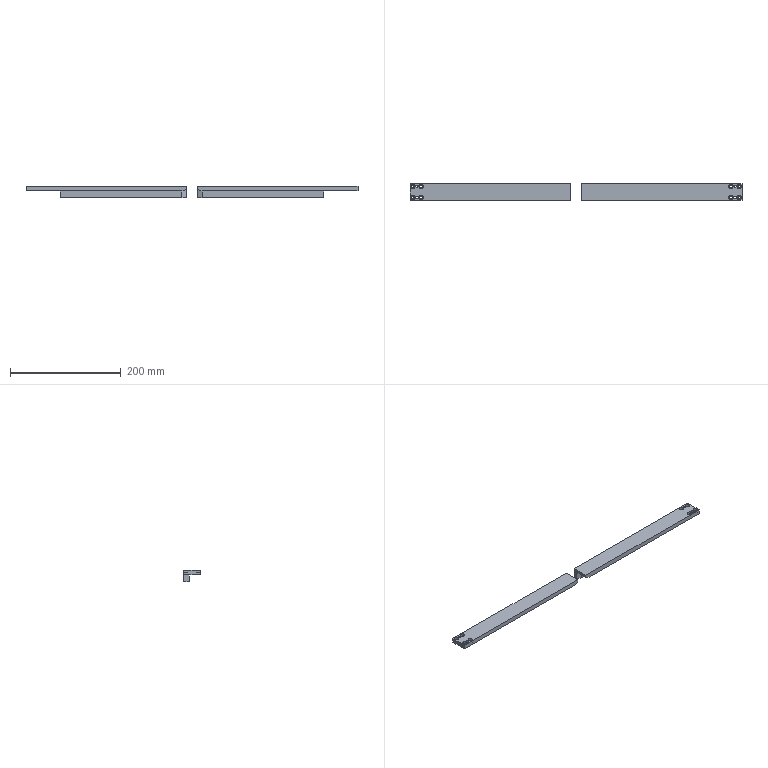NC program | NX | posted with a generic post | part box 600 x 30 x 20 mm
Whole program:
N10 G17 G21 G94 G90
(FLOOR_WALL_COPY , TOOL : D50)
N12 T01 M6
N14 G54
N16 G17 G0 G90 X-173. Y0. S6500 M3
N18 G43 Z30. H1
N20 Z7.
N22 G94 G1 Z4. F1250.
N24 X-170.
N26 X170.
N28 X173.
N30 Z7.
N32 G0 Z30.
N34 X-173.
N36 Z6.
N38 G1 Z3.
N40 X-170.
N42 X170.
N44 X173.
N46 Z6.
N48 G0 Z30.
N50 X-173.
N52 Z5.
N54 G1 Z2.
N56 X-170.
N58 X170.
N60 X173.
N62 Z5.
N64 G0 Z30.
N66 X-173.
N68 Z4.
N70 G1 Z1.
N72 X-170.
N74 X170.
N76 X173.
N78 Z4.
N80 G0 Z30.
N82 X-173.
N84 Z3.
N86 G1 Z0.
N88 X-170.
N90 X170.
N92 X173.
N94 Z3.
N96 G0 Z30.
N98 M5
(FLOOR_WALL_1 , TOOL : D10)
N100 T03 M6
N102 G54
N104 G17 G0 G90 X153.147 Y-14.991 S7000 M3
N106 G43 Z30. H3
N108 Z-8.85
N110 G94 G1 Z-11.85 F1000.
N112 X150.978
N114 X150.147 Y-17.873
N116 G2 X149.446 Y-20.147 R64. F3000.
N118 G1 X148.392
N120 G3 X150.147 Y-13.829 R63.
N122 G1 Y-8.032
N124 G2 X147.337 Y-20.147 R62.
N126 G1 X146.279
N128 G3 X149.65 Y-0.15 R61.
N130 G1 Y20.147
N132 X148.65
N134 Y-0.15
N136 G2 X145.22 Y-20.147 R60.
N138 G1 X144.158
N140 G3 X147.65 Y-0.15 R59.
N142 G1 Y20.147
N144 X146.65
N146 Y-0.15
N148 G2 X143.094 Y-20.147 R58.
N150 G1 X142.027
N152 G3 X145.65 Y-0.15 R57.
N154 G1 Y20.147
N156 X144.65
N158 Y-0.15
N160 G2 X140.958 Y-20.147 R56.
N162 G1 X139.886
N164 G3 X143.65 Y-0.15 R55.
N166 G1 Y20.147
N168 X142.65
N170 Y-0.15
N172 G2 X138.811 Y-20.147 R54.
N174 G1 X137.733
N176 G3 X141.65 Y-0.15 R53.
N178 G1 Y20.147
N180 X140.65
N182 Y-0.15
N184 G2 X136.651 Y-20.147 R52.
N186 G1 X135.566
N188 G3 X139.65 Y-0.15 R51.
N190 G1 Y20.147
N192 X138.65
N194 Y-0.15
N196 G2 X134.477 Y-20.147 R50.
N198 G1 X133.384
N200 G3 X137.65 Y-0.15 R49.
N202 G1 Y20.147
N204 X136.65
N206 Y-0.15
N208 G2 X132.286 Y-20.147 R48.
N210 G1 X131.184
N212 G3 X135.65 Y-0.15 R47.
N214 G1 Y20.147
N216 X134.65
N218 Y-0.15
N220 G2 X130.076 Y-20.147 R46.
N222 G1 X128.963
N224 G3 X133.65 Y-0.15 R45.
N226 G1 Y20.147
N228 X132.65
N230 Y-0.15
N232 G2 X127.843 Y-20.147 R44.
N234 G1 X126.717
N236 G3 X131.65 Y-0.15 R43.
N238 G1 Y20.147
N240 X130.65
N242 Y-0.15
N244 G2 X125.584 Y-20.147 R42.
N246 G1 X124.443
N248 G3 X129.65 Y-0.15 R41.
N250 G1 Y20.147
N252 X128.65
N254 Y-0.15
N256 G2 X123.293 Y-20.147 R40.
N258 G1 X122.133
N260 G3 X127.65 Y-0.15 R39.
N262 G1 Y20.147
N264 X126.65
N266 Y-0.15
N268 G2 X120.963 Y-20.147 R38.
N270 G1 X119.781
N272 G3 X125.65 Y-0.15 R37.
N274 G1 Y20.147
N276 X124.65
N278 Y-0.15
N280 G2 X118.585 Y-20.147 R36.
N282 G1 X117.375
N284 G3 X123.65 Y-0.15 R35.
N286 G1 Y20.147
N288 X122.65
N290 Y-0.15
N292 G2 X116.148 Y-20.147 R34.
N294 G1 X114.901
N296 G3 X121.65 Y-0.15 R33.
N298 G1 Y20.147
N300 X120.65
N302 Y-0.15
N304 G2 X113.632 Y-20.147 R32.
N306 G1 X112.338
N308 G3 X119.65 Y-0.15 R31.
N310 G1 Y20.147
N312 X118.65
N314 Y-0.15
N316 G2 X111.013 Y-20.147 R30.
N318 G1 X109.653
N320 G3 X117.65 Y-0.15 R29.
N322 G1 Y20.147
N324 X116.65
N326 Y-0.15
N328 G2 X108.249 Y-20.147 R28.
N330 G1 X106.792
N332 G3 X115.65 Y-0.15 R27.
N334 G1 Y20.147
N336 X114.65
N338 Y-0.15
N340 G2 X105.267 Y-20.147 R26.
N342 G1 X103.654
N344 G3 X113.65 Y-0.15 R25.
N346 G1 Y20.147
N348 X112.65
N350 Y-0.15
N352 G2 X101.921 Y-20.147 R24.
N354 G1 X100.013
N356 G3 X111.65 Y-0.15 R23.
N358 G1 Y20.147
N360 X110.65
N362 Y-0.15
N364 G2 X97.822 Y-20.147 R22.
N366 G1 X95.062
N368 G3 X109.65 Y-0.15 R21.
N370 G1 Y20.147
N372 X108.65
N374 Y-0.15
N376 G2 X88.996 Y-20.147 R20.
N378 G1 X85.997 Y-20.199
N380 Y-23.147
N382 Z-8.85
N384 G0 Z30.
N386 X-153.147 Y-18.991
N388 Z-8.85
N390 G1 Z-11.85 F1000.
N392 X-150.147 Y-20.083
N394 X-149.972 Y-20.147 F3000.
N396 X-147.048
N398 X-150.147 Y-19.019
N400 Y-17.955
N402 X-144.848 Y-19.884
N404 G3 X-144.078 Y-20.147 R21.
N406 G1 X-138.012
N408 G2 X-144.506 Y-18.944 R20.
N410 G1 X-150.147 Y-16.891
N412 Y-15.827
N414 X-144.164 Y-18.004
N416 G3 X-137.666 Y-19.15 R19.
N418 G1 X88.65
N420 G3 X107.65 Y-0.15 R19.
N422 G1 Y20.147
N424 X106.65
N426 Y-0.15
N428 G2 X88.65 Y-18.15 R18.
N430 G1 X-137.666
N432 G2 X-143.822 Y-17.064 R18.
N434 G1 X-150.147 Y-14.762
N436 Y-13.698
N438 X-143.48 Y-16.125
N440 G3 X-137.666 Y-17.15 R17.
N442 G1 X88.65
N444 G3 X105.65 Y-0.15 R17.
N446 G1 Y20.147
N448 X104.65
N450 Y-0.15
N452 G2 X88.65 Y-16.15 R16.
N454 G1 X-137.666
N456 G2 X-143.138 Y-15.185 R16.
N458 G1 X-150.147 Y-12.634
N460 Y-11.57
N462 X-142.796 Y-14.245
N464 G3 X-137.666 Y-15.15 R15.
N466 G1 X88.65
N468 G3 X103.65 Y-0.15 R15.
N470 G1 Y20.147
N472 X102.65
N474 Y-0.15
N476 G2 X88.65 Y-14.15 R14.
N478 G1 X-137.666
N480 G2 X-142.454 Y-13.306 R14.
N482 G1 X-150.147 Y-10.506
N484 Y-9.441
N486 X-142.112 Y-12.366
N488 G3 X-137.666 Y-13.15 R13.
N490 G1 X88.65
N492 G3 X101.65 Y-0.15 R13.
N494 G1 Y20.147
N496 X100.65
N498 Y-0.15
N500 G2 X88.65 Y-12.15 R12.
N502 G1 X-137.666
N504 G2 X-141.77 Y-11.426 R12.
N506 G1 X-150.147 Y-8.377
N508 Y-7.313
N510 X-141.428 Y-10.487
N512 G3 X-137.666 Y-11.15 R11.
N514 G1 X88.65
N516 G3 X99.65 Y-0.15 R11.
N518 G1 Y20.147
N520 X98.65
N522 Y-0.15
N524 G2 X88.65 Y-10.15 R10.
N526 G1 X-137.666
N528 G2 X-141.086 Y-9.547 R10.
N530 G1 X-150.147 Y-6.249
N532 Y-5.185
N534 X-140.744 Y-8.607
N536 G3 X-137.666 Y-9.15 R9.
N538 G1 X88.65
N540 G3 X97.65 Y-0.15 R9.
N542 G1 Y20.147
N544 X96.65
N546 Y-0.15
N548 G2 X88.65 Y-8.15 R8.
N550 G1 X-137.666
N552 G2 X-140.402 Y-7.668 R8.
N554 G1 X-150.147 Y-4.121
N556 Y-3.056
N558 X-140.06 Y-6.728
N560 G3 X-137.666 Y-7.15 R7.
N562 G1 X88.65
N564 G3 X95.65 Y-0.15 R7.
N566 G1 Y20.147
N568 X94.65
N570 Y-0.15
N572 G2 X88.65 Y-6.15 R6.
N574 G1 X-137.666
N576 G2 X-139.718 Y-5.788 R6.
N578 G1 X-150.147 Y-1.992
N580 Y-0.928
N582 X-139.376 Y-4.848
N584 G3 X-137.666 Y-5.15 R5.
N586 G1 X88.65
N588 G3 X93.65 Y-0.15 R5.
N590 G1 Y20.147
N592 X92.65
N594 Y-0.15
N596 G2 X88.65 Y-4.15 R4.
N598 G1 X-137.666
N600 G2 X-139.034 Y-3.909 R4.
N602 G1 X-150.147 Y0.136
N604 Y1.2
N606 X-138.692 Y-2.969
N608 G3 X-137.666 Y-3.15 R3.
N610 G1 X88.65
N612 G3 X91.65 Y-0.15 R3.
N614 G1 Y20.147
N616 X90.65
N618 Y-0.15
N620 G2 X88.65 Y-2.15 R2.
N622 G1 X-137.666
N624 G2 X-138.35 Y-2.029 R2.
N626 G1 X-150.147 Y2.264
N628 Y3.329
N630 X-138.008 Y-1.09
N632 G3 X-137.666 Y-1.15 R1.
N634 G1 X88.65
N636 G3 X89.65 Y-0.15 R1.
N638 G1 Y20.147
N640 X88.65
N642 Y-0.15
N644 X-137.666
N646 X-150.147 Y4.393
N648 X-153.15 Y5.486
N650 Z-8.85
N652 G0 Z30.
N654 M5
(FLOOR_WALL_1_COPY_1 , TOOL : D10JING)
N656 T04 M6
N658 G54
N660 G17 G0 G90 X151.139 Y-20.974 S7000 M3
N662 G43 Z30. H4
N664 Z-10.5
N666 G94 G1 Z-12. F1000.
N668 X150.865 Y-20.499
N670 G3 X149.999 Y-19.999 R1.
N672 G1 X-149.999
N674 Y-15.571
N676 X149.999
N678 Y-11.142
N680 X-149.999
N682 Y-6.714
N684 X149.999
N686 Y-2.286
N688 X-149.999
N690 Y2.142
N692 X-144.987
N694 Z-10.5
N696 G0 Z30.
N698 X94.971 Y19.999
N700 Z-10.4
N702 G1 X89. Z-12.
N704 Y2.142
N706 X149.999
N708 Y6.571
N710 X89.
N712 Y10.999
N714 X149.999
N716 Y15.427
N718 X89.
N720 G3 X89.5 Y14.561 R1.
N722 G1 Z-10.5
N724 G0 Z-8.9
N726 G1 X90.098 Y21.499 F6000.
N728 G0 Z-10.5
N730 G1 Z-12. F1000.
N732 X89. Y20.865
N734 G3 X88.5 Y19.999 R1.
N736 G1 Y0.
N738 X-137.639
N740 X-149.999 Y4.499
N742 G3 X-150.984 Y4.325 R1.
N744 G1 X-151.5 Y3.892
N746 Z-10.5
N748 G0 Z30.
N750 M5
(ZLEVEL_PROFILE_COPY_COPY_1_COPY_COPY_COPY_1_COPY_COPY , TOOL : D6R0.5)
N752 T20 M6
N754 G54
N756 G17 G0 G90 X-139.958 Y-16.121 S7000 M3
N758 G43 Z30. H20
N760 Z-12.034
N762 G94 G1 X-139.738 Y-15.994 F1000.
N764 G3 X-139.439 Y-15.474 R0.6
N766 G1 X-139.44 Y-15. F3000.
N768 Y2.784
N770 X-139.534 Y2.818 Z-12.068
N772 Y-15.
N774 X-139.533 Y-15.474
N776 X-139.581 Y-15.475 Z-12.086
N778 X-139.627 Z-12.103
N780 X-139.628 Y-15.
N782 Y2.852
N784 X-139.722 Y2.886 Z-12.137
N786 Y-15.
N788 X-139.721 Y-15.476
N790 X-139.769 Z-12.154
N792 X-139.815 Z-12.171
N794 X-139.816 Y-15.
N796 Y2.92
N798 X-139.91 Y2.955 Z-12.205
N800 Y-15.
N802 X-139.909 Y-15.477
N804 X-139.957 Z-12.222
N806 X-140.003 Z-12.239
N808 X-140.004 Y-15.
N810 Y2.989
N812 X-140.097 Y3.023 Z-12.274
N814 Y-15.
N816 Y-15.478
N818 X-140.144 Z-12.291
N820 X-140.191 Y-15.479 Z-12.308
N822 Y-15.
N824 Y3.057
N826 X-140.285 Y3.092 Z-12.342
N828 Y-15.
N830 Y-15.479
N832 X-140.332 Y-15.48 Z-12.359
N834 X-140.379 Z-12.376
N836 Y-15.
N838 Y3.126
N840 X-140.473 Y3.16 Z-12.41
N842 Y-15.
N844 Y-15.48
N846 X-140.52 Y-15.481 Z-12.428
N848 X-140.567 Z-12.445
N850 Y-15.
N852 Y3.194
N854 X-140.661 Y3.228 Z-12.479
N856 Y-15.
N858 Y-15.482
N860 X-140.708 Z-12.496
N862 X-140.755 Z-12.513
N864 Y-15.
N866 Y3.263
N868 X-140.849 Y3.297 Z-12.547
N870 Y-15.
N872 Y-15.483
N874 X-140.896 Z-12.564
N876 X-140.943 Y-15.484 Z-12.581
N878 Y-15.
N880 Y3.331
N882 X-141.037 Y3.365 Z-12.616
N884 Y-15.
N886 Y-15.484
N888 X-141.084 Z-12.633
N890 X-141.131 Y-15.485 Z-12.65
N892 Y-15.
N894 Y3.399
N896 X-141.225 Y3.434 Z-12.684
N898 Y-15.
N900 Y-15.485
N902 X-141.272 Z-12.701
N904 X-141.319 Y-15.486 Z-12.718
N906 Y-15.
N908 Y3.468
N910 X-141.413 Y3.502 Z-12.752
N912 Y-15.
N914 Y-15.486
N916 X-141.46 Z-12.77
N918 X-141.506 Z-12.787
N920 X-141.507 Y-15.
N922 Y3.536
N924 X-141.601 Y3.57 Z-12.821
N926 Y-15.
N928 X-141.6 Y-15.487
N930 X-141.648 Z-12.838
N932 X-141.694 Z-12.855
N934 X-141.695 Y-15.
N936 Y3.605
N938 X-141.789 Y3.639 Z-12.889
N940 Y-15.
N942 X-141.788 Y-15.487
N944 X-141.836 Y-15.488 Z-12.906
N946 X-141.882 Z-12.923
N948 X-141.883 Y-15.
N950 Y3.673
N952 X-141.977 Y3.707 Z-12.958
N954 Y-15.
N956 X-141.976 Y-15.488
N958 X-142.024 Z-12.975
N960 X-142.07 Y-15.489 Z-12.992
N962 X-142.071 Y-15.
N964 Y3.741
N966 X-142.165 Y3.776 Z-13.026
N968 Y-15.
N970 X-142.164 Y-15.489
N972 X-142.212 Z-13.043
N974 X-142.258 Z-13.06
N976 X-142.259 Y-15.
N978 Y3.81
N980 X-142.353 Y3.844 Z-13.094
N982 Y-15.
N984 X-142.352 Y-15.49
N986 X-142.4 Z-13.112
N988 X-142.446 Z-13.129
N990 X-142.447 Y-15.
N992 Y3.878
N994 X-142.541 Y3.912 Z-13.163
N996 Y-15.
N998 X-142.54 Y-15.491
N1000 X-142.588 Z-13.18
N1002 X-142.634 Z-13.197
N1004 X-142.635 Y-15.
N1006 Y3.947
N1008 X-142.729 Y3.981 Z-13.231
N1010 Y-15.
N1012 X-142.728 Y-15.491
N1014 X-142.776 Z-13.248
N1016 X-142.822 Z-13.265
N1018 X-142.823 Y-15.
N1020 Y4.015
N1022 X-142.917 Y4.049 Z-13.3
N1024 Y-15.
N1026 X-142.916 Y-15.491
N1028 X-142.964 Z-13.317
N1030 X-143.01 Z-13.334
N1032 X-143.011 Y-15.
N1034 Y4.083
N1036 X-143.105 Y4.118 Z-13.368
N1038 Y-15.
N1040 X-143.104 Y-15.491
N1042 X-143.151 Z-13.385
N1044 X-143.198 Z-13.402
N1046 Y-15.
N1048 Y4.152
N1050 X-143.292 Y4.186 Z-13.436
N1052 Y-15.
N1054 Y-15.491
N1056 X-143.339 Z-13.454
N1058 X-143.386 Z-13.471
N1060 Y-15.
N1062 Y4.22
N1064 X-143.48 Y4.254 Z-13.505
N1066 Y-15.
N1068 Y-15.491
N1070 X-143.527 Z-13.522
N1072 X-143.574 Z-13.539
N1074 Y-15.
N1076 Y4.289
N1078 X-143.668 Y4.323 Z-13.573
N1080 Y-15.
N1082 Y-15.491
N1084 X-143.715 Z-13.59
N1086 X-143.762 Z-13.607
N1088 Y-15.
N1090 Y4.357
N1092 X-143.856 Y4.391 Z-13.642
N1094 Y-15.
N1096 Y-15.491
N1098 X-143.903 Z-13.659
N1100 X-143.95 Z-13.676
N1102 Y-15.
N1104 Y4.425
N1106 X-144.044 Y4.46 Z-13.71
N1108 Y-15.
N1110 Y-15.491
N1112 X-144.091 Z-13.727
N1114 X-144.138 Z-13.744
N1116 Y-15.
N1118 Y4.494
N1120 X-144.232 Y4.528 Z-13.779
N1122 Y-15.
N1124 Y-15.491
N1126 X-144.279 Z-13.796
N1128 X-144.326 Z-13.813
N1130 Y-15.
N1132 Y4.562
N1134 X-144.42 Y4.596 Z-13.847
N1136 Y-15.
N1138 Y-15.491
N1140 X-144.467 Z-13.864
N1142 X-144.514 Z-13.881
N1144 Y-15.
N1146 Y4.631
N1148 X-144.608 Y4.665 Z-13.915
N1150 Y-15.
N1152 Y-15.49
N1154 X-144.655 Z-13.932
N1156 X-144.701 Z-13.95
N1158 X-144.702 Y-15.
N1160 Y4.699
N1162 X-144.796 Y4.733 Z-13.984
N1164 Y-15.
N1166 X-144.795 Y-15.49
N1168 X-144.843 Y-15.489 Z-14.001
N1170 X-144.889 Z-14.018
N1172 X-144.89 Y-15.
N1174 Y4.767
N1176 X-144.984 Y4.802 Z-14.052
N1178 Y-15.
N1180 X-144.983 Y-15.489
N1182 X-145.031 Z-14.069
N1184 X-145.077 Y-15.488 Z-14.086
N1186 X-145.078 Y-15.
N1188 Y4.836
N1190 X-145.172 Y4.87 Z-14.121
N1192 Y-15.
N1194 X-145.171 Y-15.488
N1196 X-145.219 Z-14.138
N1198 X-145.265 Z-14.155
N1200 X-145.266 Y-15.
N1202 Y4.904
N1204 X-145.36 Y4.938 Z-14.189
N1206 Y-15.
N1208 X-145.359 Y-15.487
N1210 X-145.407 Z-14.206
N1212 X-145.453 Z-14.223
N1214 X-145.454 Y-15.
N1216 Y4.973
N1218 X-145.548 Y5.007 Z-14.257
N1220 Y-15.
N1222 X-145.547 Y-15.487
N1224 X-145.595 Y-15.486 Z-14.274
N1226 X-145.641 Z-14.292
N1228 X-145.642 Y-15.
N1230 Y5.041
N1232 X-145.736 Y5.075 Z-14.326
N1234 Y-15.
N1236 X-145.735 Y-15.486
N1238 X-145.783 Z-14.343
N1240 X-145.829 Y-15.485 Z-14.36
N1242 X-145.83 Y-15.
N1244 Y5.109
N1246 X-145.924 Y5.144 Z-14.394
N1248 Y-15.
N1250 X-145.923 Y-15.485
N1252 X-145.971 Z-14.411
N1254 X-146.017 Z-14.428
N1256 X-146.018 Y-15.
N1258 Y5.178
N1260 X-146.112 Y5.214 Z-14.463
N1262 Y-15.
N1264 X-146.111 Y-15.484
N1266 X-146.159 Z-14.48
N1268 X-146.205 Y-15.483 Z-14.497
N1270 Y-15.
N1272 Y5.253
N1274 X-146.299 Y5.296 Z-14.531
N1276 Y-15.
N1278 Y-15.483
N1280 X-146.346 Y-15.482 Z-14.548
N1282 X-146.393 Z-14.565
N1284 Y-15.
N1286 Y5.343
N1288 X-146.487 Y5.395 Z-14.599
N1290 Y-15.
N1292 Y-15.482
N1294 X-146.534 Y-15.481 Z-14.616
N1296 X-146.581 Z-14.634
N1298 Y-15.
N1300 Y5.451
N1302 X-146.675 Y5.511 Z-14.668
N1304 Y-15.
N1306 Y-15.48
N1308 X-146.722 Z-14.685
N1310 X-146.769 Z-14.702
N1312 Y-15.
N1314 Y5.577
N1316 X-146.863 Y5.649 Z-14.736
N1318 Y-15.
N1320 Y-15.479
N1322 X-146.91 Z-14.753
N1324 X-146.957 Y-15.478 Z-14.77
N1326 Y-15.
N1328 Y5.726
N1330 X-147.051 Y5.811 Z-14.805
N1332 Y-15.
N1334 Y-15.478
N1336 X-147.098 Y-15.477 Z-14.822
N1338 X-147.144 Z-14.839
N1340 X-147.145 Y-15.
N1342 Y5.903
N1344 X-147.239 Y6.003 Z-14.873
N1346 Y-15.
N1348 X-147.238 Y-15.476
N1350 X-147.286 Z-14.89
N1352 X-147.332 Z-14.907
N1354 X-147.333 Y-15.
N1356 Y6.114
N1358 X-147.427 Y6.237 Z-14.941
N1360 Y-15.
N1362 X-147.426 Y-15.475
N1364 X-147.474 Z-14.958
N1366 X-147.52 Z-14.976
N1368 X-147.521 Y-15.
N1370 Y6.374
N1372 X-147.57 Y6.452 Z-14.993
N1374 X-147.615 Y6.53 Z-15.01
N1376 Y-15.
N1378 X-147.614 Y-15.474
N1380 X-147.662 Z-15.027
N1382 X-147.708 Y-15.473 Z-15.044
N1384 X-147.709 Y6.572
N1386 X-147.798 Y6.918
N1388 X-147.839 Y7.032 Z-15.055
N1390 X-147.876 Y7.147 Z-15.067
N1392 X-147.908 Y7.263 Z-15.078
N1394 X-147.803 Y6.918
N1396 X-147.802 Y-15.473
N1398 X-147.85 Y-15.472 Z-15.095
N1400 X-147.896 Z-15.112
N1402 X-147.897 Y6.918
N1404 X-147.908 Y7.263
N1406 X-147.941 Y7.41 Z-15.119
N1408 X-147.967 Y7.557 Z-15.126
N1410 X-147.985 Y7.705 Z-15.133
N1412 X-147.996 Y7.852 Z-15.14
N1414 X-148. Y8. Z-15.147
N1416 X-147.991 Y7.762
N1418 X-147.99 Y-15.465
N1420 X-148.038 Y-15.365 Z-15.164
N1422 X-148.084 Y-15.264 Z-15.181
N1424 X-148.085 Y8.646
N1426 G3 X-148.385 Y9.165 R0.6
N1428 G1 X-148.61 Y9.295
N1430 G0 Z30.
N1432 M5
(ZLEVEL_PROFILE_COPY_1_COPY_COPY_COPY_COPY_2_COPY_COPY , TOOL : D6A45)
N1434 T02 M6
N1436 G54
N1438 G17 G0 G90 X-145.92 Y16.95 S7000 M3
N1440 G43 Z30. H2
N1442 Z-1.
N1444 G94 G1 X-145.521 Y16.259 F1000.
N1446 G3 X-145.001 Y15.959 R0.6
N1448 G1 X83.501
N1450 G2 X84.459 Y15.001 R0.958
N1452 G1 Y4.999
N1454 G2 X83.501 Y4.041 R0.958
N1456 G1 X-136.758
N1458 G2 X-137.085 Y4.099 R0.954
N1460 G1 X-145.329 Y7.1
N1462 G2 X-145.959 Y7.999 R0.957
N1464 G1 Y15.001
N1466 G2 X-145.001 Y15.959 R0.966
N1468 G3 X-144.484 Y16.263 R0.6
N1470 G1 X-143.976 Y17.159
N1472 G0 Z30.
(ZLEVEL_PROFILE_COPY_1_COPY_COPY_COPY_COPY_2_COPY_COPY_COPY , TOOL : D6A45)
N1474 X125.042 Y10.081
N1476 Z-13.
N1478 G1 X125.52 Y10.991
N1480 G3 X125. Y11.291 R0.6
N1482 X123.709 Y10. R1.291
N1484 X125. Y11.291 R-1.291
N1486 X124.48 Y10.991 R0.6
N1488 G1 X124.958 Y10.081
N1490 G0 Z30.
N1492 X140.042
N1494 Z-13.
N1496 G1 X140.52 Y10.991
N1498 G3 X140. Y11.291 R0.6
N1500 X138.709 Y10. R1.291
N1502 X140. Y11.291 R-1.291
N1504 X139.48 Y10.991 R0.6
N1506 G1 X139.958 Y10.081
N1508 G0 Z30.
N1510 Y-10.081
N1512 Z-13.
N1514 G1 X139.48 Y-10.991
N1516 G3 X140. Y-11.291 R0.6
N1518 X141.291 Y-10. R1.291
N1520 X140. Y-11.291 R-1.291
N1522 X140.52 Y-10.991 R0.6
N1524 G1 X140.042 Y-10.081
N1526 G0 Z30.
N1528 X124.958
N1530 Z-13.
N1532 G1 X124.48 Y-10.991
N1534 G3 X125. Y-11.291 R0.6
N1536 X126.291 Y-10. R1.291
N1538 X125. Y-11.291 R-1.291
N1540 X125.52 Y-10.991 R0.6
N1542 G1 X125.042 Y-10.081
N1544 G0 Z30.
N1546 X131.459 Y-9.5
N1548 Z-12.
N1550 G1 Z-13.
N1552 Y-10.5
N1554 G3 X132.5 Y-11.541 R1.041
N1556 X133.541 Y-10.5 R1.041
N1558 G1 Y-9.5
N1560 G3 X132.5 Y-8.459 R1.041
N1562 X131.459 Y-9.5 R1.041
N1564 X131.759 Y-10.02 R0.6
N1566 G0 Z30.
N1568 X132.5 Y11.041
N1570 Z-12.
N1572 G1 Z-13.
N1574 G3 X131.459 Y10. R1.041
N1576 X132.5 Y11.041 R-1.041
N1578 X131.98 Y10.741 R0.6
N1580 G0 Z30.
N1582 X87.023 Y17.159
N1584 Z-13.
N1586 G1 X86.405 Y16.109
N1588 G3 X86.665 Y15.959 R0.3
N1590 G1 X145.001
N1592 G2 X145.959 Y15.001 R0.958
N1594 G1 Y-15.001
N1596 G2 X145.001 Y-15.959 R0.958
N1598 G1 X-136.758
N1600 G3 X-137.278 Y-16.259 R0.6
N1602 G1 X-137.681 Y-16.957
N1604 G0 Z30.
N1606 M5
N1608 M2